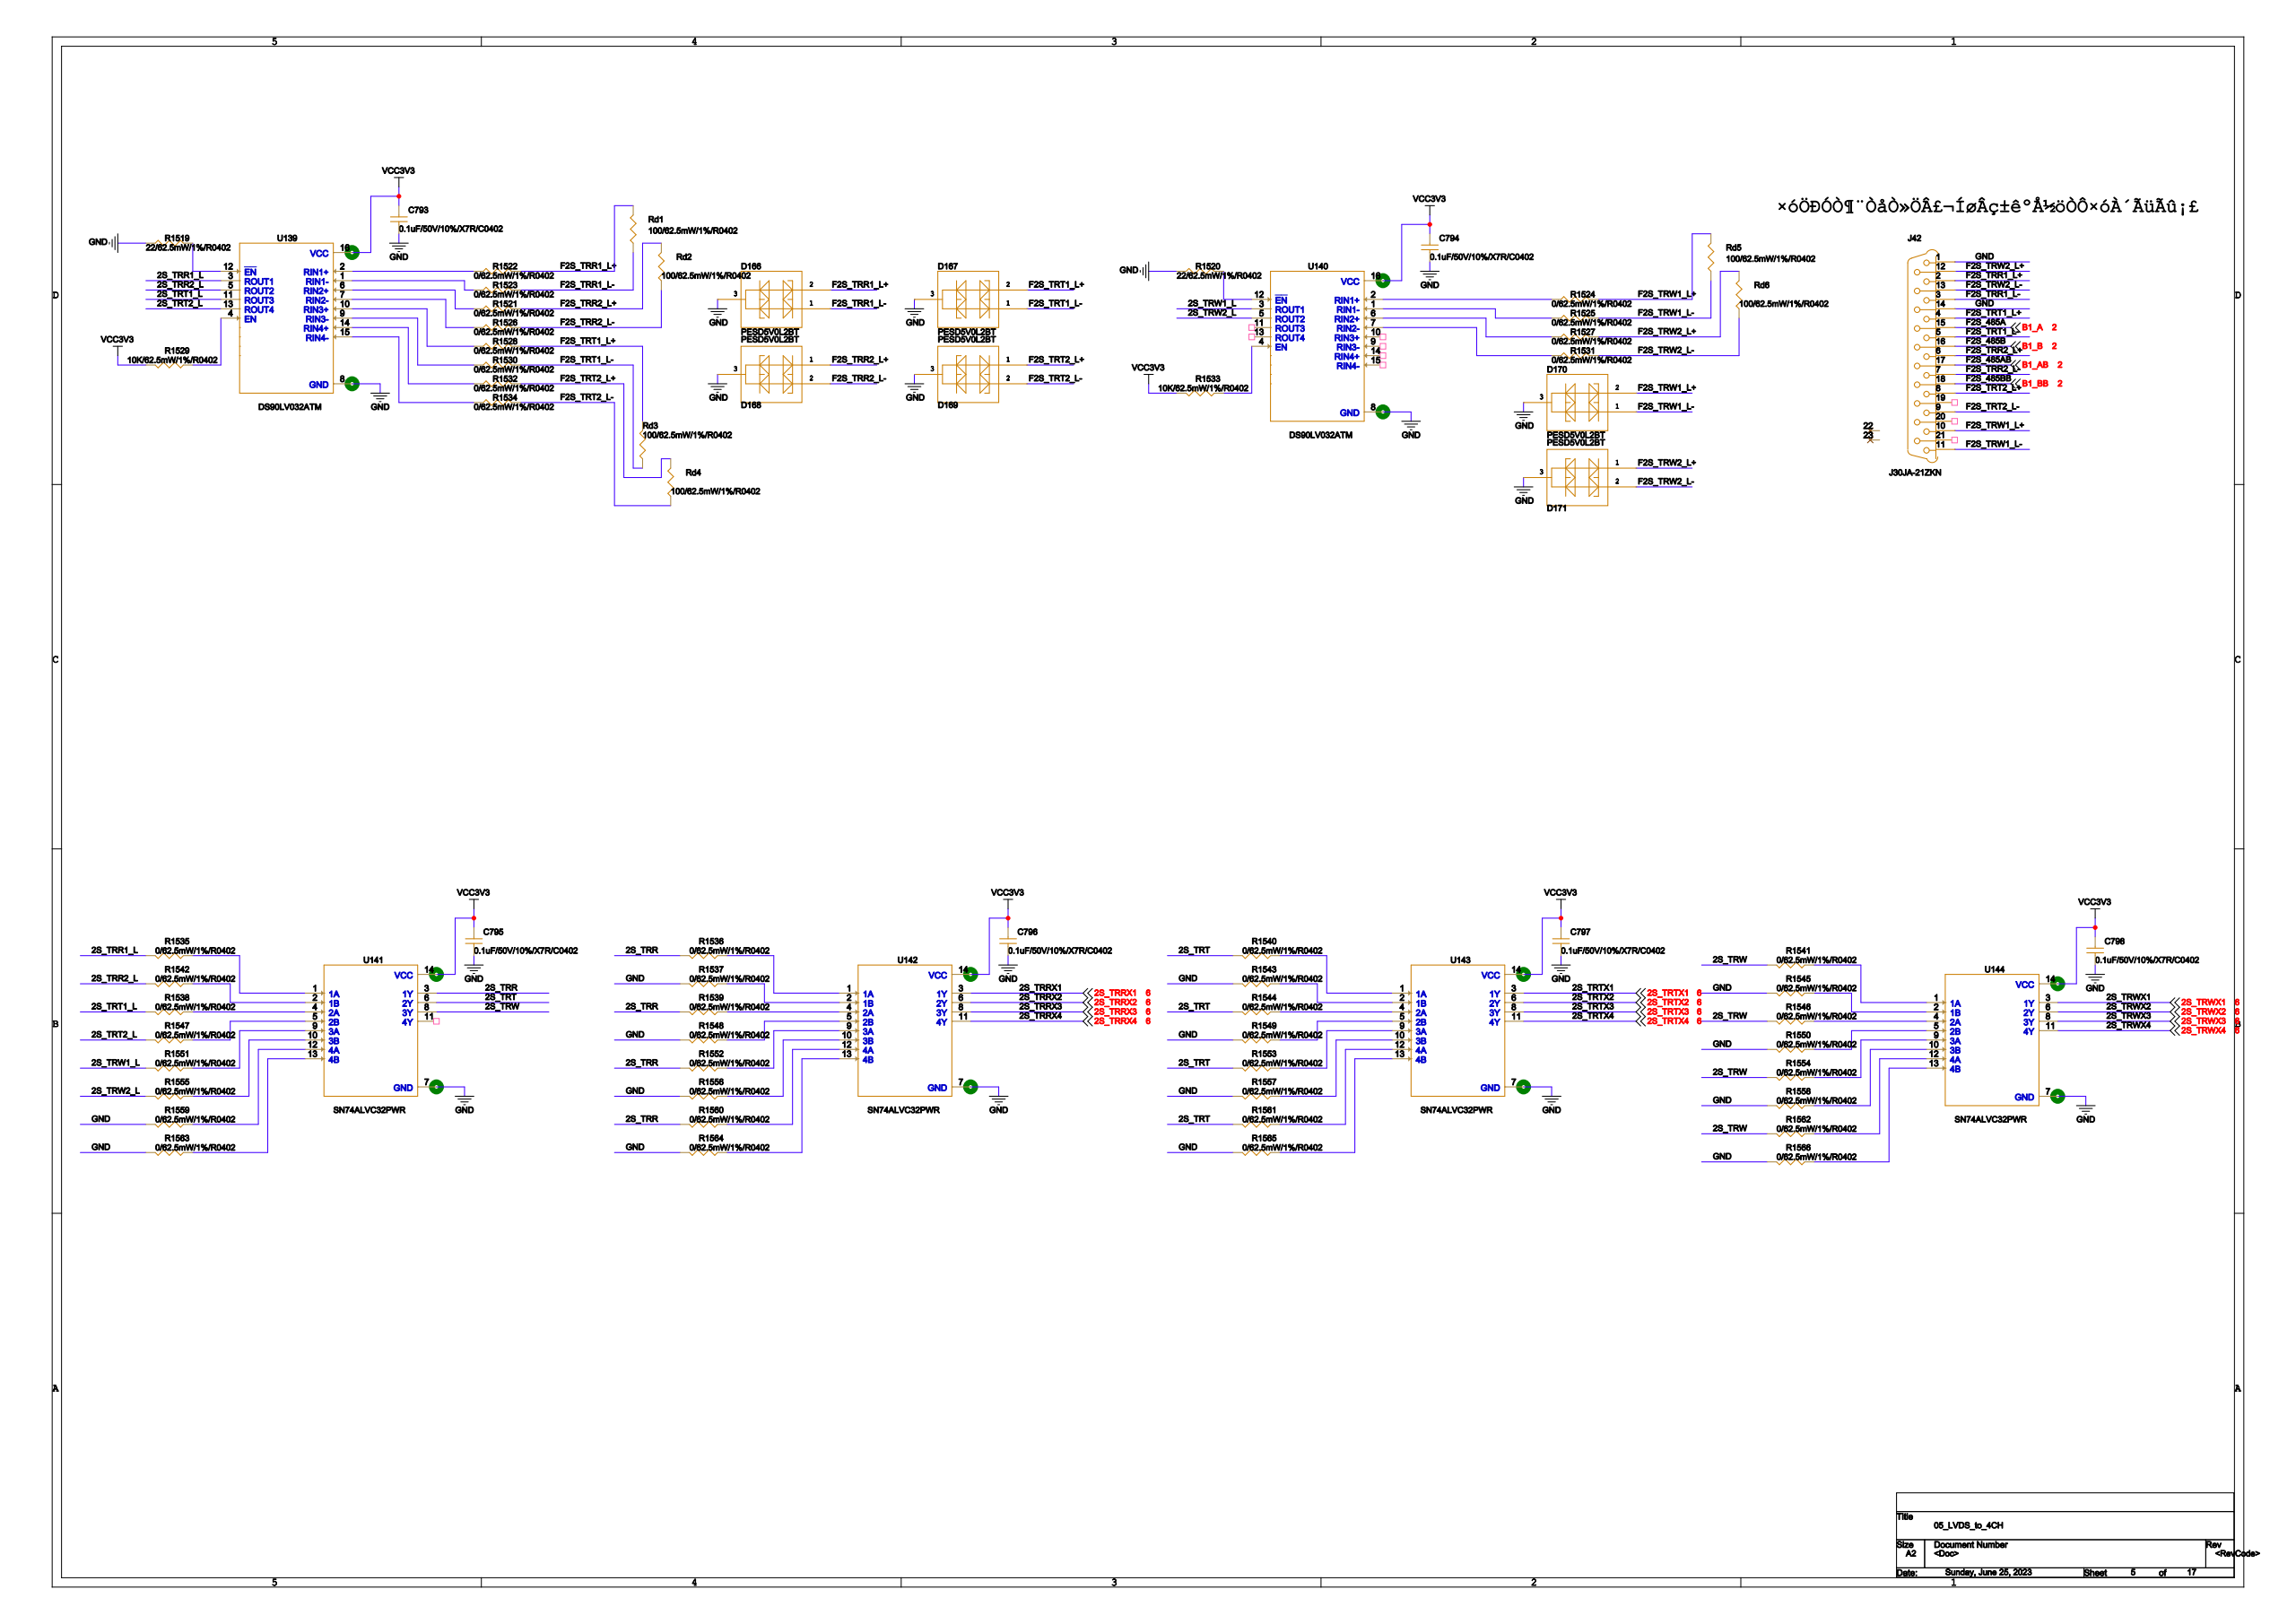Circuit board | Cadence Allegro | 2002 parts | 1538 nets | one sheet of the schematic
Parts on this sheet (reference | value | footprint):
C793 | 0.1uF/50V/10%/X7R/C0402 | 0402
C794 | 0.1uF/50V/10%/X7R/C0402 | 0402
C795 | 0.1uF/50V/10%/X7R/C0402 | 0402
C796 | 0.1uF/50V/10%/X7R/C0402 | 0402
C797 | 0.1uF/50V/10%/X7R/C0402 | 0402
C798 | 0.1uF/50V/10%/X7R/C0402 | 0402
D166 | PESD5V0L2BT | SOT23
D167 | PESD5V0L2BT | SOT23
D168 | PESD5V0L2BT | SOT23
D169 | PESD5V0L2BT | SOT23
D170 | PESD5V0L2BT | SOT23
D171 | PESD5V0L2BT | SOT23
J42 | J30JA-21ZKN | J30JA-21ZKN
R1519 | 22/62.5mW/1%/R0402 | 0402
R1520 | 22/62.5mW/1%/R0402 | 0402
R1521 | 0/62.5mW/1%/R0402 | 0402
R1522 | 0/62.5mW/1%/R0402 | 0402
R1523 | 0/62.5mW/1%/R0402 | 0402
R1524 | 0/62.5mW/1%/R0402 | 0402
R1525 | 0/62.5mW/1%/R0402 | 0402
R1526 | 0/62.5mW/1%/R0402 | 0402
R1527 | 0/62.5mW/1%/R0402 | 0402
R1528 | 0/62.5mW/1%/R0402 | 0402
R1529 | 10K/62.5mW/1%/R0402 | 0402
R1530 | 0/62.5mW/1%/R0402 | 0402
R1531 | 0/62.5mW/1%/R0402 | 0402
R1532 | 0/62.5mW/1%/R0402 | 0402
R1533 | 10K/62.5mW/1%/R0402 | 0402
R1534 | 0/62.5mW/1%/R0402 | 0402
R1535 | 0/62.5mW/1%/R0402 | 0402
R1536 | 0/62.5mW/1%/R0402 | 0402
R1537 | 0/62.5mW/1%/R0402 | 0402
R1538 | 0/62.5mW/1%/R0402 | 0402
R1539 | 0/62.5mW/1%/R0402 | 0402
R1540 | 0/62.5mW/1%/R0402 | 0402
R1541 | 0/62.5mW/1%/R0402 | 0402
R1542 | 0/62.5mW/1%/R0402 | 0402
R1543 | 0/62.5mW/1%/R0402 | 0402
R1544 | 0/62.5mW/1%/R0402 | 0402
R1545 | 0/62.5mW/1%/R0402 | 0402
R1546 | 0/62.5mW/1%/R0402 | 0402
R1547 | 0/62.5mW/1%/R0402 | 0402
R1548 | 0/62.5mW/1%/R0402 | 0402
R1549 | 0/62.5mW/1%/R0402 | 0402
R1550 | 0/62.5mW/1%/R0402 | 0402
R1551 | 0/62.5mW/1%/R0402 | 0402
R1552 | 0/62.5mW/1%/R0402 | 0402
R1553 | 0/62.5mW/1%/R0402 | 0402
R1554 | 0/62.5mW/1%/R0402 | 0402
R1555 | 0/62.5mW/1%/R0402 | 0402
R1556 | 0/62.5mW/1%/R0402 | 0402
R1557 | 0/62.5mW/1%/R0402 | 0402
R1558 | 0/62.5mW/1%/R0402 | 0402
R1559 | 0/62.5mW/1%/R0402 | 0402
R1560 | 0/62.5mW/1%/R0402 | 0402
R1561 | 0/62.5mW/1%/R0402 | 0402
R1562 | 0/62.5mW/1%/R0402 | 0402
R1563 | 0/62.5mW/1%/R0402 | 0402
R1564 | 0/62.5mW/1%/R0402 | 0402
R1565 | 0/62.5mW/1%/R0402 | 0402
R1566 | 0/62.5mW/1%/R0402 | 0402
U139 | DS90LV032ATM | SOIC127P600X175-16N
U140 | DS90LV032ATM | SOIC127P600X175-16N
U141 | SN74ALVC32PWR | SOP65P640X120-14N
U142 | SN74ALVC32PWR | SOP65P640X120-14N
U143 | SN74ALVC32PWR | SOP65P640X120-14N
U144 | SN74ALVC32PWR | SOP65P640X120-14N
Nets of these parts (net: part-pin ...):
3.3V: C793-1 C794-1 C795-1 C796-1 C797-1 C798-1 R1529-1 R1533-1 U139-16 U140-16 U141-14 U142-14 U143-14 U144-14
AGND: C793-2 C794-2 C795-2 C796-2 C797-2 C798-2 D166-3 D167-3 D168-3 D169-3 D170-3 D171-3 J42-1 J42-14 R1519-2 R1520-2 R1537-1 R1543-1 R1545-1 R1548-1 R1549-1 R1550-1 R1556-1 R1557-1 R1558-1 R1559-1 R1563-1 R1564-1 R1565-1 R1566-1 U139-8 U140-8 U141-7 U142-7 U143-7 U144-7
F2S_TRW1_L+: D170-2 J42-10 R1524-1
F2S_TRW1_L-: D170-1 J42-11 R1525-1
F2S_TRW2_L+: D171-1 J42-12 R1527-1
F2S_TRW2_L-: D171-2 J42-13 R1531-1
B1_A: J42-15
B1_B: J42-16
B1_AB: J42-17
B1_BB: J42-18
F2S_TRR1_L+: D166-2 J42-2 R1522-1
F2S_TRR1_L-: D166-1 J42-3 R1523-1
F2S_TRT1_L+: D167-2 J42-4 R1528-1
F2S_TRT1_L-: D167-1 J42-5 R1530-1
F2S_TRR2_L+: D168-1 J42-6 R1521-1
F2S_TRR2_L-: D168-2 J42-7 R1526-1
F2S_TRT2_L+: D169-1 J42-8 R1532-1
F2S_TRT2_L-: D169-2 J42-9 R1534-1
N23932818: R1521-2 U139-6
N23932828: R1522-2 U139-2
N23932816: R1523-2 U139-1
N23933318: R1524-2 U140-2
N23933306: R1525-2 U140-1
N23932814: R1526-2 U139-7
N23933308: R1527-2 U140-6
N23932880: R1528-2 U139-10
N23932860: R1530-2 U139-9
N23933304: R1531-2 U140-7
N23932862: R1532-2 U139-14
N23932858: R1534-2 U139-15
2S_TRR1_L: R1535-1 U139-3
N23947474: R1535-2 U141-1
2S_TRR: R1536-1 R1539-1 R1552-1 R1560-1 U141-3
N23951252: R1536-2 U142-1
N23951246: R1537-2 U142-2
2S_TRT1_L: R1538-1 U139-11
N23947464: R1538-2 U141-4
N23951241: R1539-2 U142-4
2S_TRT: R1540-1 R1544-1 R1553-1 R1561-1 U141-6
N23952028: R1540-2 U143-1
2S_TRW: R1541-1 R1546-1 R1554-1 R1562-1 U141-8
N23952637: R1541-2 U144-1
2S_TRR2_L: R1542-1 U139-5
N23947468: R1542-2 U141-2
N23952022: R1543-2 U143-2
N23952017: R1544-2 U143-4
N23952631: R1545-2 U144-2
N23952626: R1546-2 U144-4
2S_TRT2_L: R1547-1 U139-13
N23947458: R1547-2 U141-5
N23951235: R1548-2 U142-5
N23952011: R1549-2 U143-5
N23952620: R1550-2 U144-5
2S_TRW1_L: R1551-1 U140-3
N23947916: R1551-2 U141-9
N23951299: R1552-2 U142-9
N23952075: R1553-2 U143-9
N23952684: R1554-2 U144-9
2S_TRW2_L: R1555-1 U140-5
N23947925: R1555-2 U141-10
N23951313: R1556-2 U142-10
N23952089: R1557-2 U143-10
N23952698: R1558-2 U144-10
N23948082: R1559-2 U141-12
N23951333: R1560-2 U142-12
N23952098: R1561-2 U143-12
N23952707: R1562-2 U144-12
N23948113: R1563-2 U141-13
N23951346: R1564-2 U142-13
N23952119: R1565-2 U143-13
N23952728: R1566-2 U144-13
2S_TRRX1: U142-3
2S_TRTX1: U143-3
2S_TRWX1: U144-3
2S_TRRX2: U142-6
2S_TRTX2: U143-6
2S_TRWX2: U144-6
2S_TRRX3: U142-8
2S_TRTX3: U143-8
2S_TRWX3: U144-8
2S_TRRX4: U142-11
2S_TRTX4: U143-11
2S_TRWX4: U144-11
N23932768: R1529-2 U139-4
N23932772: R1519-1 U139-12
N23933268: R1533-2 U140-4
N23933272: R1520-1 U140-12